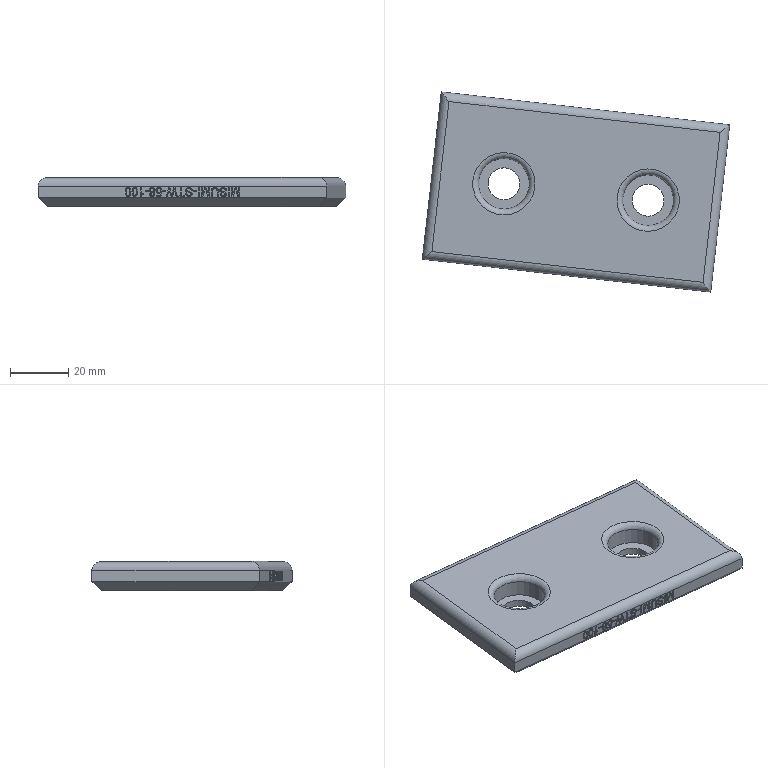Part | NX | features XQ 2 | 1 solid | 159 faces | box 105.923 x 68.947 x 10 mm | volume 51823 mm3 | plane 109 | spline 40 | cylinder 8 | torus 2 | commonest cylinder face diameters 6 x4 11 x2 17.5 x2